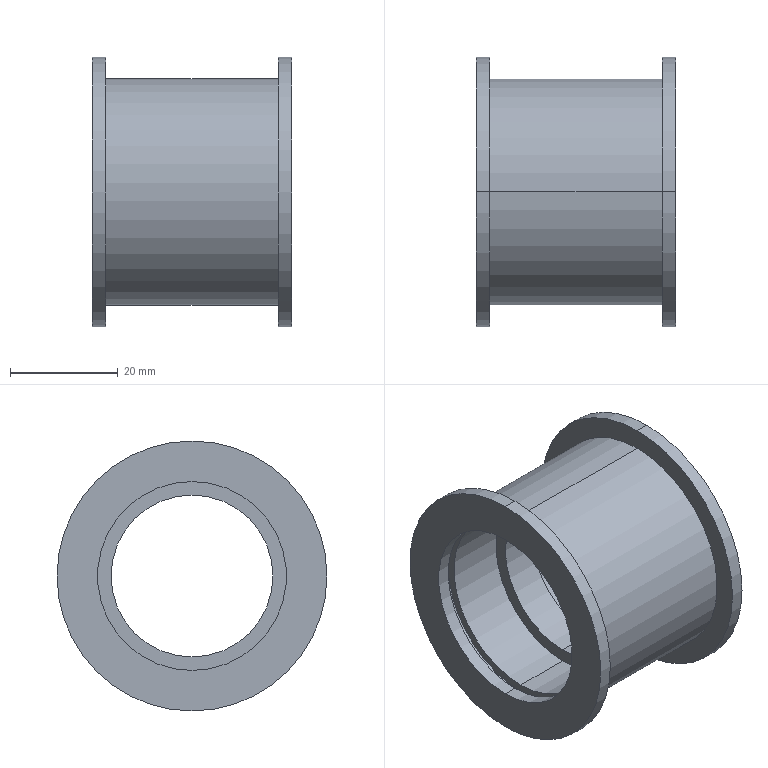Part | SolidWorks | features ICE 5, Fillet 2, MirrorPattern 2, CirPattern 1, Extrusion 1, RevCut 1 | 1 solid | 30 faces | box 37 x 50 x 50 mm | volume 19824 mm3 | cylinder 20 | plane 10 | commonest cylinder face diameters 35 x8 38 x4 50 x4 30 x2 42 x2
STEP:
#1=CARTESIAN_POINT('',(16.,0.,-19.));
#2=VERTEX_POINT('',#1);
#3=CARTESIAN_POINT('',(16.,0.,19.));
#4=VERTEX_POINT('',#3);
#5=CARTESIAN_POINT('',(16.,0.,0.));
#6=DIRECTION('',(1.,0.,0.));
#7=DIRECTION('',(0.,0.,-1.));
#8=AXIS2_PLACEMENT_3D('',#5,#6,#7);
#9=CIRCLE('',#8,19.);
#10=EDGE_CURVE('',#2,#4,#9,.T.);
#11=ORIENTED_EDGE('',*,*,#10,.T.);
#12=CARTESIAN_POINT('',(14.5,0.,19.));
#13=VERTEX_POINT('',#12);
#14=CARTESIAN_POINT('',(0.,0.,19.));
#15=DIRECTION('',(-1.,0.,0.));
#16=VECTOR('',#15,1000.);
#17=LINE('',#14,#16);
#18=EDGE_CURVE('',#4,#13,#17,.T.);
#19=ORIENTED_EDGE('',*,*,#18,.T.);
#20=CARTESIAN_POINT('',(14.5,0.,-19.));
#21=VERTEX_POINT('',#20);
#22=CARTESIAN_POINT('',(14.5,0.,0.));
#23=DIRECTION('',(1.,0.,0.));
#24=DIRECTION('',(0.,0.,-1.));
#25=AXIS2_PLACEMENT_3D('',#22,#23,#24);
#26=CIRCLE('',#25,19.);
#27=EDGE_CURVE('',#21,#13,#26,.T.);
#28=ORIENTED_EDGE('',*,*,#27,.F.);
#29=CARTESIAN_POINT('',(0.,0.,-19.));
#30=DIRECTION('',(-1.,0.,0.));
#31=VECTOR('',#30,1000.);
#32=LINE('',#29,#31);
#33=EDGE_CURVE('',#2,#21,#32,.T.);
#34=ORIENTED_EDGE('',*,*,#33,.F.);
#35=EDGE_LOOP('',(#11,#19,#28,#34));
#36=FACE_OUTER_BOUND('',#35,.T.);
#37=CARTESIAN_POINT('',(0.,0.,0.));
#38=DIRECTION('',(-1.,0.,0.));
#39=DIRECTION('',(0.,0.,-1.));
#40=AXIS2_PLACEMENT_3D('',#37,#38,#39);
#41=CYLINDRICAL_SURFACE('',#40,19.);
#42=ADVANCED_FACE('',(#36),#41,.F.);
#43=CARTESIAN_POINT('',(3.5,0.,-17.5));
#44=VERTEX_POINT('',#43);
#45=CARTESIAN_POINT('',(3.5,0.,17.5));
#46=VERTEX_POINT('',#45);
#47=CARTESIAN_POINT('',(3.5,0.,0.));
#48=DIRECTION('',(-1.,0.,0.));
#49=DIRECTION('',(0.,0.,1.));
#50=AXIS2_PLACEMENT_3D('',#47,#48,#49);
#51=CIRCLE('',#50,17.5);
#52=EDGE_CURVE('',#44,#46,#51,.T.);
#53=ORIENTED_EDGE('',*,*,#52,.T.);
#54=CARTESIAN_POINT('',(14.5,0.,17.5));
#55=VERTEX_POINT('',#54);
#56=CARTESIAN_POINT('',(3.5,0.,17.5));
#57=DIRECTION('',(1.,0.,0.));
#58=VECTOR('',#57,1000.);
#59=LINE('',#56,#58);
#60=EDGE_CURVE('',#46,#55,#59,.T.);
#61=ORIENTED_EDGE('',*,*,#60,.T.);
#62=CARTESIAN_POINT('',(14.5,0.,-17.5));
#63=VERTEX_POINT('',#62);
#64=CARTESIAN_POINT('',(14.5,0.,0.));
#65=DIRECTION('',(1.,0.,0.));
#66=DIRECTION('',(0.,0.,-1.));
#67=AXIS2_PLACEMENT_3D('',#64,#65,#66);
#68=CIRCLE('',#67,17.5);
#69=EDGE_CURVE('',#55,#63,#68,.T.);
#70=ORIENTED_EDGE('',*,*,#69,.T.);
#71=CARTESIAN_POINT('',(3.5,0.,-17.5));
#72=DIRECTION('',(1.,0.,0.));
#73=VECTOR('',#72,1000.);
#74=LINE('',#71,#73);
#75=EDGE_CURVE('',#44,#63,#74,.T.);
#76=ORIENTED_EDGE('',*,*,#75,.F.);
#77=EDGE_LOOP('',(#53,#61,#70,#76));
#78=FACE_OUTER_BOUND('',#77,.T.);
#79=CARTESIAN_POINT('',(3.5,0.,0.));
#80=DIRECTION('',(1.,0.,0.));
#81=DIRECTION('',(0.,0.,-1.));
#82=AXIS2_PLACEMENT_3D('',#79,#80,#81);
#83=CYLINDRICAL_SURFACE('',#82,17.5);
#84=ADVANCED_FACE('',(#78),#83,.F.);
#85=CARTESIAN_POINT('',(-16.,0.,19.));
#86=VERTEX_POINT('',#85);
#87=CARTESIAN_POINT('',(-16.,0.,-19.));
#88=VERTEX_POINT('',#87);
#89=CARTESIAN_POINT('',(-16.,0.,0.));
#90=DIRECTION('',(1.,0.,0.));
#91=DIRECTION('',(0.,0.,-1.));
#92=AXIS2_PLACEMENT_3D('',#89,#90,#91);
#93=CIRCLE('',#92,19.);
#94=EDGE_CURVE('',#86,#88,#93,.T.);
#95=ORIENTED_EDGE('',*,*,#94,.F.);
#96=CARTESIAN_POINT('',(-14.5,0.,19.));
#97=VERTEX_POINT('',#96);
#98=CARTESIAN_POINT('',(0.,0.,19.));
#99=DIRECTION('',(1.,0.,0.));
#100=VECTOR('',#99,1000.);
#101=LINE('',#98,#100);
#102=EDGE_CURVE('',#86,#97,#101,.T.);
#103=ORIENTED_EDGE('',*,*,#102,.T.);
#104=CARTESIAN_POINT('',(-14.5,0.,-19.));
#105=VERTEX_POINT('',#104);
#106=CARTESIAN_POINT('',(-14.5,0.,0.));
#107=DIRECTION('',(1.,0.,0.));
#108=DIRECTION('',(0.,0.,-1.));
#109=AXIS2_PLACEMENT_3D('',#106,#107,#108);
#110=CIRCLE('',#109,19.);
#111=EDGE_CURVE('',#97,#105,#110,.T.);
#112=ORIENTED_EDGE('',*,*,#111,.T.);
#113=CARTESIAN_POINT('',(0.,0.,-19.));
#114=DIRECTION('',(1.,0.,0.));
#115=VECTOR('',#114,1000.);
#116=LINE('',#113,#115);
#117=EDGE_CURVE('',#88,#105,#116,.T.);
#118=ORIENTED_EDGE('',*,*,#117,.F.);
#119=EDGE_LOOP('',(#95,#103,#112,#118));
#120=FACE_OUTER_BOUND('',#119,.T.);
#121=CARTESIAN_POINT('',(0.,0.,0.));
#122=DIRECTION('',(1.,0.,0.));
#123=DIRECTION('',(0.,0.,-1.));
#124=AXIS2_PLACEMENT_3D('',#121,#122,#123);
#125=CYLINDRICAL_SURFACE('',#124,19.);
#126=ADVANCED_FACE('',(#120),#125,.F.);
#127=CARTESIAN_POINT('',(-3.5,0.,-17.5));
#128=VERTEX_POINT('',#127);
#129=CARTESIAN_POINT('',(-3.5,0.,17.5));
#130=VERTEX_POINT('',#129);
#131=CARTESIAN_POINT('',(-3.5,0.,0.));
#132=DIRECTION('',(-1.,0.,0.));
#133=DIRECTION('',(0.,0.,1.));
#134=AXIS2_PLACEMENT_3D('',#131,#132,#133);
#135=CIRCLE('',#134,17.5);
#136=EDGE_CURVE('',#128,#130,#135,.T.);
#137=ORIENTED_EDGE('',*,*,#136,.F.);
#138=CARTESIAN_POINT('',(-14.5,0.,-17.5));
#139=VERTEX_POINT('',#138);
#140=CARTESIAN_POINT('',(-3.5,0.,-17.5));
#141=DIRECTION('',(-1.,0.,0.));
#142=VECTOR('',#141,1000.);
#143=LINE('',#140,#142);
#144=EDGE_CURVE('',#128,#139,#143,.T.);
#145=ORIENTED_EDGE('',*,*,#144,.T.);
#146=CARTESIAN_POINT('',(-14.5,0.,17.5));
#147=VERTEX_POINT('',#146);
#148=CARTESIAN_POINT('',(-14.5,0.,0.));
#149=DIRECTION('',(1.,0.,0.));
#150=DIRECTION('',(0.,0.,-1.));
#151=AXIS2_PLACEMENT_3D('',#148,#149,#150);
#152=CIRCLE('',#151,17.5);
#153=EDGE_CURVE('',#147,#139,#152,.T.);
#154=ORIENTED_EDGE('',*,*,#153,.F.);
#155=CARTESIAN_POINT('',(-3.5,0.,17.5));
#156=DIRECTION('',(-1.,0.,0.));
#157=VECTOR('',#156,1000.);
#158=LINE('',#155,#157);
#159=EDGE_CURVE('',#130,#147,#158,.T.);
#160=ORIENTED_EDGE('',*,*,#159,.F.);
#161=EDGE_LOOP('',(#137,#145,#154,#160));
#162=FACE_OUTER_BOUND('',#161,.T.);
#163=CARTESIAN_POINT('',(-3.5,0.,0.));
#164=DIRECTION('',(-1.,0.,0.));
#165=DIRECTION('',(0.,0.,1.));
#166=AXIS2_PLACEMENT_3D('',#163,#164,#165);
#167=CYLINDRICAL_SURFACE('',#166,17.5);
#168=ADVANCED_FACE('',(#162),#167,.F.);
#169=CARTESIAN_POINT('',(-18.5,0.,-25.));
#170=VERTEX_POINT('',#169);
#171=CARTESIAN_POINT('',(-18.5,0.,25.));
#172=VERTEX_POINT('',#171);
#173=CARTESIAN_POINT('',(-18.5,0.,0.));
#174=DIRECTION('',(1.,0.,0.));
#175=DIRECTION('',(0.,0.,-1.));
#176=AXIS2_PLACEMENT_3D('',#173,#174,#175);
#177=CIRCLE('',#176,25.);
#178=EDGE_CURVE('',#170,#172,#177,.T.);
#179=ORIENTED_EDGE('',*,*,#178,.T.);
#180=CARTESIAN_POINT('',(-16.,0.,25.));
#181=VERTEX_POINT('',#180);
#182=CARTESIAN_POINT('',(-17.5,0.,25.));
#183=DIRECTION('',(1.,0.,0.));
#184=VECTOR('',#183,1000.);
#185=LINE('',#182,#184);
#186=EDGE_CURVE('',#172,#181,#185,.T.);
#187=ORIENTED_EDGE('',*,*,#186,.T.);
#188=CARTESIAN_POINT('',(-16.,0.,-25.));
#189=VERTEX_POINT('',#188);
#190=CARTESIAN_POINT('',(-16.,0.,0.));
#191=DIRECTION('',(1.,0.,0.));
#192=DIRECTION('',(0.,0.,-1.));
#193=AXIS2_PLACEMENT_3D('',#190,#191,#192);
#194=CIRCLE('',#193,25.);
#195=EDGE_CURVE('',#189,#181,#194,.T.);
#196=ORIENTED_EDGE('',*,*,#195,.F.);
#197=CARTESIAN_POINT('',(-17.5,0.,-25.));
#198=DIRECTION('',(1.,0.,0.));
#199=VECTOR('',#198,1000.);
#200=LINE('',#197,#199);
#201=EDGE_CURVE('',#170,#189,#200,.T.);
#202=ORIENTED_EDGE('',*,*,#201,.F.);
#203=EDGE_LOOP('',(#179,#187,#196,#202));
#204=FACE_OUTER_BOUND('',#203,.T.);
#205=CARTESIAN_POINT('',(-17.5,0.,0.));
#206=DIRECTION('',(1.,0.,0.));
#207=DIRECTION('',(0.,0.,-1.));
#208=AXIS2_PLACEMENT_3D('',#205,#206,#207);
#209=CYLINDRICAL_SURFACE('',#208,25.);
#210=ADVANCED_FACE('',(#204),#209,.T.);
#211=CARTESIAN_POINT('',(18.5,0.,-25.));
#212=VERTEX_POINT('',#211);
#213=CARTESIAN_POINT('',(18.5,0.,25.));
#214=VERTEX_POINT('',#213);
#215=CARTESIAN_POINT('',(18.5,0.,0.));
#216=DIRECTION('',(1.,0.,0.));
#217=DIRECTION('',(0.,0.,-1.));
#218=AXIS2_PLACEMENT_3D('',#215,#216,#217);
#219=CIRCLE('',#218,25.);
#220=EDGE_CURVE('',#212,#214,#219,.T.);
#221=ORIENTED_EDGE('',*,*,#220,.F.);
#222=CARTESIAN_POINT('',(16.,0.,-25.));
#223=VERTEX_POINT('',#222);
#224=CARTESIAN_POINT('',(17.5,0.,-25.));
#225=DIRECTION('',(-1.,0.,0.));
#226=VECTOR('',#225,1000.);
#227=LINE('',#224,#226);
#228=EDGE_CURVE('',#212,#223,#227,.T.);
#229=ORIENTED_EDGE('',*,*,#228,.T.);
#230=CARTESIAN_POINT('',(16.,0.,25.));
#231=VERTEX_POINT('',#230);
#232=CARTESIAN_POINT('',(16.,0.,0.));
#233=DIRECTION('',(1.,0.,0.));
#234=DIRECTION('',(0.,0.,-1.));
#235=AXIS2_PLACEMENT_3D('',#232,#233,#234);
#236=CIRCLE('',#235,25.);
#237=EDGE_CURVE('',#223,#231,#236,.T.);
#238=ORIENTED_EDGE('',*,*,#237,.T.);
#239=CARTESIAN_POINT('',(17.5,0.,25.));
#240=DIRECTION('',(-1.,0.,0.));
#241=VECTOR('',#240,1000.);
#242=LINE('',#239,#241);
#243=EDGE_CURVE('',#214,#231,#242,.T.);
#244=ORIENTED_EDGE('',*,*,#243,.F.);
#245=EDGE_LOOP('',(#221,#229,#238,#244));
#246=FACE_OUTER_BOUND('',#245,.T.);
#247=CARTESIAN_POINT('',(17.5,0.,0.));
#248=DIRECTION('',(-1.,0.,0.));
#249=DIRECTION('',(0.,0.,1.));
#250=AXIS2_PLACEMENT_3D('',#247,#248,#249);
#251=CYLINDRICAL_SURFACE('',#250,25.);
#252=ADVANCED_FACE('',(#246),#251,.T.);
#253=CARTESIAN_POINT('',(16.,0.,-21.));
#254=VERTEX_POINT('',#253);
#255=CARTESIAN_POINT('',(16.,0.,21.));
#256=VERTEX_POINT('',#255);
#257=CARTESIAN_POINT('',(16.,0.,0.));
#258=DIRECTION('',(1.,0.,0.));
#259=DIRECTION('',(0.,0.,-1.));
#260=AXIS2_PLACEMENT_3D('',#257,#258,#259);
#261=CIRCLE('',#260,21.);
#262=EDGE_CURVE('',#254,#256,#261,.T.);
#263=ORIENTED_EDGE('',*,*,#262,.F.);
#264=CARTESIAN_POINT('',(-16.,0.,-21.));
#265=VERTEX_POINT('',#264);
#266=CARTESIAN_POINT('',(16.,0.,-21.));
#267=DIRECTION('',(-1.,0.,0.));
#268=VECTOR('',#267,1000.);
#269=LINE('',#266,#268);
#270=EDGE_CURVE('',#254,#265,#269,.T.);
#271=ORIENTED_EDGE('',*,*,#270,.T.);
#272=CARTESIAN_POINT('',(-16.,0.,21.));
#273=VERTEX_POINT('',#272);
#274=CARTESIAN_POINT('',(-16.,0.,0.));
#275=DIRECTION('',(-1.,0.,0.));
#276=DIRECTION('',(0.,0.,1.));
#277=AXIS2_PLACEMENT_3D('',#274,#275,#276);
#278=CIRCLE('',#277,21.);
#279=EDGE_CURVE('',#273,#265,#278,.T.);
#280=ORIENTED_EDGE('',*,*,#279,.F.);
#281=CARTESIAN_POINT('',(16.,0.,21.));
#282=DIRECTION('',(-1.,0.,0.));
#283=VECTOR('',#282,1000.);
#284=LINE('',#281,#283);
#285=EDGE_CURVE('',#256,#273,#284,.T.);
#286=ORIENTED_EDGE('',*,*,#285,.F.);
#287=EDGE_LOOP('',(#263,#271,#280,#286));
#288=FACE_OUTER_BOUND('',#287,.T.);
#289=CARTESIAN_POINT('',(16.,0.,0.));
#290=DIRECTION('',(-1.,0.,0.));
#291=DIRECTION('',(0.,0.,1.));
#292=AXIS2_PLACEMENT_3D('',#289,#290,#291);
#293=CYLINDRICAL_SURFACE('',#292,21.);
#294=ADVANCED_FACE('',(#288),#293,.T.);
#295=CARTESIAN_POINT('',(-16.,0.,17.5));
#296=VERTEX_POINT('',#295);
#297=CARTESIAN_POINT('',(-16.,0.,-17.5));
#298=VERTEX_POINT('',#297);
#299=CARTESIAN_POINT('',(-16.,0.,0.));
#300=DIRECTION('',(1.,0.,0.));
#301=DIRECTION('',(0.,0.,-1.));
#302=AXIS2_PLACEMENT_3D('',#299,#300,#301);
#303=CIRCLE('',#302,17.5);
#304=EDGE_CURVE('',#296,#298,#303,.T.);
#305=ORIENTED_EDGE('',*,*,#304,.T.);
#306=CARTESIAN_POINT('',(-18.5,0.,-17.5));
#307=VERTEX_POINT('',#306);
#308=CARTESIAN_POINT('',(-3.5,0.,-17.5));
#309=DIRECTION('',(-1.,0.,0.));
#310=VECTOR('',#309,1000.);
#311=LINE('',#308,#310);
#312=EDGE_CURVE('',#298,#307,#311,.T.);
#313=ORIENTED_EDGE('',*,*,#312,.T.);
#314=CARTESIAN_POINT('',(-18.5,0.,17.5));
#315=VERTEX_POINT('',#314);
#316=CARTESIAN_POINT('',(-18.5,0.,0.));
#317=DIRECTION('',(-1.,0.,0.));
#318=DIRECTION('',(0.,0.,1.));
#319=AXIS2_PLACEMENT_3D('',#316,#317,#318);
#320=CIRCLE('',#319,17.5);
#321=EDGE_CURVE('',#307,#315,#320,.T.);
#322=ORIENTED_EDGE('',*,*,#321,.T.);
#323=CARTESIAN_POINT('',(-3.5,0.,17.5));
#324=DIRECTION('',(-1.,0.,0.));
#325=VECTOR('',#324,1000.);
#326=LINE('',#323,#325);
#327=EDGE_CURVE('',#296,#315,#326,.T.);
#328=ORIENTED_EDGE('',*,*,#327,.F.);
#329=EDGE_LOOP('',(#305,#313,#322,#328));
#330=FACE_OUTER_BOUND('',#329,.T.);
#331=CARTESIAN_POINT('',(-3.5,0.,0.));
#332=DIRECTION('',(-1.,0.,0.));
#333=DIRECTION('',(0.,0.,1.));
#334=AXIS2_PLACEMENT_3D('',#331,#332,#333);
#335=CYLINDRICAL_SURFACE('',#334,17.5);
#336=ADVANCED_FACE('',(#330),#335,.F.);
#337=CARTESIAN_POINT('',(3.5,0.,-15.));
#338=VERTEX_POINT('',#337);
#339=CARTESIAN_POINT('',(3.5,0.,15.));
#340=VERTEX_POINT('',#339);
#341=CARTESIAN_POINT('',(3.5,0.,0.));
#342=DIRECTION('',(-1.,0.,0.));
#343=DIRECTION('',(0.,0.,-1.));
#344=AXIS2_PLACEMENT_3D('',#341,#342,#343);
#345=CIRCLE('',#344,15.);
#346=EDGE_CURVE('',#338,#340,#345,.T.);
#347=ORIENTED_EDGE('',*,*,#346,.F.);
#348=CARTESIAN_POINT('',(-3.5,0.,-15.));
#349=VERTEX_POINT('',#348);
#350=CARTESIAN_POINT('',(18.5,0.,-15.));
#351=DIRECTION('',(-1.,0.,0.));
#352=VECTOR('',#351,1000.);
#353=LINE('',#350,#352);
#354=EDGE_CURVE('',#338,#349,#353,.T.);
#355=ORIENTED_EDGE('',*,*,#354,.T.);
#356=CARTESIAN_POINT('',(-3.5,0.,15.));
#357=VERTEX_POINT('',#356);
#358=CARTESIAN_POINT('',(-3.5,0.,0.));
#359=DIRECTION('',(1.,0.,0.));
#360=DIRECTION('',(0.,0.,1.));
#361=AXIS2_PLACEMENT_3D('',#358,#359,#360);
#362=CIRCLE('',#361,15.);
#363=EDGE_CURVE('',#357,#349,#362,.T.);
#364=ORIENTED_EDGE('',*,*,#363,.F.);
#365=CARTESIAN_POINT('',(18.5,0.,15.));
#366=DIRECTION('',(-1.,0.,0.));
#367=VECTOR('',#366,1000.);
#368=LINE('',#365,#367);
#369=EDGE_CURVE('',#340,#357,#368,.T.);
#370=ORIENTED_EDGE('',*,*,#369,.F.);
#371=EDGE_LOOP('',(#347,#355,#364,#370));
#372=FACE_OUTER_BOUND('',#371,.T.);
#373=CARTESIAN_POINT('',(18.5,0.,0.));
#374=DIRECTION('',(-1.,0.,0.));
#375=DIRECTION('',(0.,0.,1.));
#376=AXIS2_PLACEMENT_3D('',#373,#374,#375);
#377=CYLINDRICAL_SURFACE('',#376,15.);
#378=ADVANCED_FACE('',(#372),#377,.F.);
#379=CARTESIAN_POINT('',(16.,0.,17.5));
#380=VERTEX_POINT('',#379);
#381=CARTESIAN_POINT('',(16.,0.,-17.5));
#382=VERTEX_POINT('',#381);
#383=CARTESIAN_POINT('',(16.,0.,0.));
#384=DIRECTION('',(1.,0.,0.));
#385=DIRECTION('',(0.,0.,-1.));
#386=AXIS2_PLACEMENT_3D('',#383,#384,#385);
#387=CIRCLE('',#386,17.5);
#388=EDGE_CURVE('',#380,#382,#387,.T.);
#389=ORIENTED_EDGE('',*,*,#388,.F.);
#390=CARTESIAN_POINT('',(18.5,0.,17.5));
#391=VERTEX_POINT('',#390);
#392=CARTESIAN_POINT('',(3.5,0.,17.5));
#393=DIRECTION('',(1.,0.,0.));
#394=VECTOR('',#393,1000.);
#395=LINE('',#392,#394);
#396=EDGE_CURVE('',#380,#391,#395,.T.);
#397=ORIENTED_EDGE('',*,*,#396,.T.);
#398=CARTESIAN_POINT('',(18.5,0.,-17.5));
#399=VERTEX_POINT('',#398);
#400=CARTESIAN_POINT('',(18.5,0.,0.));
#401=DIRECTION('',(-1.,0.,0.));
#402=DIRECTION('',(0.,0.,1.));
#403=AXIS2_PLACEMENT_3D('',#400,#401,#402);
#404=CIRCLE('',#403,17.5);
#405=EDGE_CURVE('',#399,#391,#404,.T.);
#406=ORIENTED_EDGE('',*,*,#405,.F.);
#407=CARTESIAN_POINT('',(3.5,0.,-17.5));
#408=DIRECTION('',(1.,0.,0.));
#409=VECTOR('',#408,1000.);
#410=LINE('',#407,#409);
#411=EDGE_CURVE('',#382,#399,#410,.T.);
#412=ORIENTED_EDGE('',*,*,#411,.F.);
#413=EDGE_LOOP('',(#389,#397,#406,#412));
#414=FACE_OUTER_BOUND('',#413,.T.);
#415=CARTESIAN_POINT('',(3.5,0.,0.));
#416=DIRECTION('',(1.,0.,0.));
#417=DIRECTION('',(0.,0.,-1.));
#418=AXIS2_PLACEMENT_3D('',#415,#416,#417);
#419=CYLINDRICAL_SURFACE('',#418,17.5);
#420=ADVANCED_FACE('',(#414),#419,.F.);
#421=ORIENTED_EDGE('',*,*,#396,.F.);
#422=CARTESIAN_POINT('',(16.,0.,0.));
#423=DIRECTION('',(1.,0.,0.));
#424=DIRECTION('',(0.,0.,-1.));
#425=AXIS2_PLACEMENT_3D('',#422,#423,#424);
#426=CIRCLE('',#425,17.5);
#427=EDGE_CURVE('',#382,#380,#426,.T.);
#428=ORIENTED_EDGE('',*,*,#427,.F.);
#429=ORIENTED_EDGE('',*,*,#411,.T.);
#430=CARTESIAN_POINT('',(18.5,0.,0.));
#431=DIRECTION('',(-1.,0.,0.));
#432=DIRECTION('',(0.,0.,1.));
#433=AXIS2_PLACEMENT_3D('',#430,#431,#432);
#434=CIRCLE('',#433,17.5);
#435=EDGE_CURVE('',#391,#399,#434,.T.);
#436=ORIENTED_EDGE('',*,*,#435,.F.);
#437=EDGE_LOOP('',(#421,#428,#429,#436));
#438=FACE_OUTER_BOUND('',#437,.T.);
#439=CARTESIAN_POINT('',(3.5,0.,0.));
#440=DIRECTION('',(1.,0.,0.));
#441=DIRECTION('',(0.,0.,-1.));
#442=AXIS2_PLACEMENT_3D('',#439,#440,#441);
#443=CYLINDRICAL_SURFACE('',#442,17.5);
#444=ADVANCED_FACE('',(#438),#443,.F.);
#445=ORIENTED_EDGE('',*,*,#354,.F.);
#446=CARTESIAN_POINT('',(3.5,0.,0.));
#447=DIRECTION('',(-1.,0.,0.));
#448=DIRECTION('',(0.,0.,-1.));
#449=AXIS2_PLACEMENT_3D('',#446,#447,#448);
#450=CIRCLE('',#449,15.);
#451=EDGE_CURVE('',#340,#338,#450,.T.);
#452=ORIENTED_EDGE('',*,*,#451,.F.);
#453=ORIENTED_EDGE('',*,*,#369,.T.);
#454=CARTESIAN_POINT('',(-3.5,0.,0.));
#455=DIRECTION('',(1.,0.,0.));
#456=DIRECTION('',(0.,0.,1.));
#457=AXIS2_PLACEMENT_3D('',#454,#455,#456);
#458=CIRCLE('',#457,15.);
#459=EDGE_CURVE('',#349,#357,#458,.T.);
#460=ORIENTED_EDGE('',*,*,#459,.F.);
#461=EDGE_LOOP('',(#445,#452,#453,#460));
#462=FACE_OUTER_BOUND('',#461,.T.);
#463=CARTESIAN_POINT('',(18.5,0.,0.));
#464=DIRECTION('',(-1.,0.,0.));
#465=DIRECTION('',(0.,0.,1.));
#466=AXIS2_PLACEMENT_3D('',#463,#464,#465);
#467=CYLINDRICAL_SURFACE('',#466,15.);
#468=ADVANCED_FACE('',(#462),#467,.F.);
#469=CARTESIAN_POINT('',(18.5,0.,0.));
#470=DIRECTION('',(1.,0.,0.));
#471=DIRECTION('',(0.,0.,-1.));
#472=AXIS2_PLACEMENT_3D('',#469,#470,#471);
#473=CIRCLE('',#472,25.);
#474=EDGE_CURVE('',#214,#212,#473,.T.);
#475=ORIENTED_EDGE('',*,*,#474,.T.);
#476=ORIENTED_EDGE('',*,*,#220,.T.);
#477=EDGE_LOOP('',(#475,#476));
#478=FACE_OUTER_BOUND('',#477,.T.);
#479=ORIENTED_EDGE('',*,*,#405,.T.);
#480=ORIENTED_EDGE('',*,*,#435,.T.);
#481=EDGE_LOOP('',(#479,#480));
#482=FACE_BOUND('',#481,.T.);
#483=CARTESIAN_POINT('',(18.5,0.,0.));
#484=DIRECTION('',(1.,0.,0.));
#485=DIRECTION('',(0.,0.,-1.));
#486=AXIS2_PLACEMENT_3D('',#483,#484,#485);
#487=PLANE('',#486);
#488=ADVANCED_FACE('',(#478,#482),#487,.T.);
#489=ORIENTED_EDGE('',*,*,#312,.F.);
#490=CARTESIAN_POINT('',(-16.,0.,0.));
#491=DIRECTION('',(1.,0.,0.));
#492=DIRECTION('',(0.,0.,-1.));
#493=AXIS2_PLACEMENT_3D('',#490,#491,#492);
#494=CIRCLE('',#493,17.5);
#495=EDGE_CURVE('',#298,#296,#494,.T.);
#496=ORIENTED_EDGE('',*,*,#495,.T.);
#497=ORIENTED_EDGE('',*,*,#327,.T.);
#498=CARTESIAN_POINT('',(-18.5,0.,0.));
#499=DIRECTION('',(-1.,0.,0.));
#500=DIRECTION('',(0.,0.,1.));
#501=AXIS2_PLACEMENT_3D('',#498,#499,#500);
#502=CIRCLE('',#501,17.5);
#503=EDGE_CURVE('',#315,#307,#502,.T.);
#504=ORIENTED_EDGE('',*,*,#503,.T.);
#505=EDGE_LOOP('',(#489,#496,#497,#504));
#506=FACE_OUTER_BOUND('',#505,.T.);
#507=CARTESIAN_POINT('',(-3.5,0.,0.));
#508=DIRECTION('',(-1.,0.,0.));
#509=DIRECTION('',(0.,0.,1.));
#510=AXIS2_PLACEMENT_3D('',#507,#508,#509);
#511=CYLINDRICAL_SURFACE('',#510,17.5);
#512=ADVANCED_FACE('',(#506),#511,.F.);
#513=ORIENTED_EDGE('',*,*,#270,.F.);
#514=CARTESIAN_POINT('',(16.,0.,0.));
#515=DIRECTION('',(1.,0.,0.));
#516=DIRECTION('',(0.,0.,-1.));
#517=AXIS2_PLACEMENT_3D('',#514,#515,#516);
#518=CIRCLE('',#517,21.);
#519=EDGE_CURVE('',#256,#254,#518,.T.);
#520=ORIENTED_EDGE('',*,*,#519,.F.);
#521=ORIENTED_EDGE('',*,*,#285,.T.);
#522=CARTESIAN_POINT('',(-16.,0.,0.));
#523=DIRECTION('',(-1.,0.,0.));
#524=DIRECTION('',(0.,0.,1.));
#525=AXIS2_PLACEMENT_3D('',#522,#523,#524);
#526=CIRCLE('',#525,21.);
#527=EDGE_CURVE('',#265,#273,#526,.T.);
#528=ORIENTED_EDGE('',*,*,#527,.F.);
#529=EDGE_LOOP('',(#513,#520,#521,#528));
#530=FACE_OUTER_BOUND('',#529,.T.);
#531=CARTESIAN_POINT('',(16.,0.,0.));
#532=DIRECTION('',(-1.,0.,0.));
#533=DIRECTION('',(0.,0.,1.));
#534=AXIS2_PLACEMENT_3D('',#531,#532,#533);
#535=CYLINDRICAL_SURFACE('',#534,21.);
#536=ADVANCED_FACE('',(#530),#535,.T.);
#537=CARTESIAN_POINT('',(16.,0.,0.));
#538=DIRECTION('',(1.,0.,0.));
#539=DIRECTION('',(0.,0.,-1.));
#540=AXIS2_PLACEMENT_3D('',#537,#538,#539);
#541=CIRCLE('',#540,25.);
#542=EDGE_CURVE('',#231,#223,#541,.T.);
#543=ORIENTED_EDGE('',*,*,#542,.F.);
#544=ORIENTED_EDGE('',*,*,#237,.F.);
#545=EDGE_LOOP('',(#543,#544));
#546=FACE_OUTER_BOUND('',#545,.T.);
#547=ORIENTED_EDGE('',*,*,#519,.T.);
#548=ORIENTED_EDGE('',*,*,#262,.T.);
#549=EDGE_LOOP('',(#547,#548));
#550=FACE_BOUND('',#549,.T.);
#551=CARTESIAN_POINT('',(16.,0.,0.));
#552=DIRECTION('',(1.,0.,0.));
#553=DIRECTION('',(0.,0.,-1.));
#554=AXIS2_PLACEMENT_3D('',#551,#552,#553);
#555=PLANE('',#554);
#556=ADVANCED_FACE('',(#546,#550),#555,.F.);
#557=ORIENTED_EDGE('',*,*,#228,.F.);
#558=ORIENTED_EDGE('',*,*,#474,.F.);
#559=ORIENTED_EDGE('',*,*,#243,.T.);
#560=ORIENTED_EDGE('',*,*,#542,.T.);
#561=EDGE_LOOP('',(#557,#558,#559,#560));
#562=FACE_OUTER_BOUND('',#561,.T.);
#563=CARTESIAN_POINT('',(17.5,0.,0.));
#564=DIRECTION('',(-1.,0.,0.));
#565=DIRECTION('',(0.,0.,1.));
#566=AXIS2_PLACEMENT_3D('',#563,#564,#565);
#567=CYLINDRICAL_SURFACE('',#566,25.);
#568=ADVANCED_FACE('',(#562),#567,.T.);
#569=ORIENTED_EDGE('',*,*,#195,.T.);
#570=CARTESIAN_POINT('',(-16.,0.,0.));
#571=DIRECTION('',(1.,0.,0.));
#572=DIRECTION('',(0.,0.,-1.));
#573=AXIS2_PLACEMENT_3D('',#570,#571,#572);
#574=CIRCLE('',#573,25.);
#575=EDGE_CURVE('',#181,#189,#574,.T.);
#576=ORIENTED_EDGE('',*,*,#575,.T.);
#577=EDGE_LOOP('',(#569,#576));
#578=FACE_OUTER_BOUND('',#577,.T.);
#579=ORIENTED_EDGE('',*,*,#279,.T.);
#580=ORIENTED_EDGE('',*,*,#527,.T.);
#581=EDGE_LOOP('',(#579,#580));
#582=FACE_BOUND('',#581,.T.);
#583=CARTESIAN_POINT('',(-16.,0.,0.));
#584=DIRECTION('',(-1.,0.,0.));
#585=DIRECTION('',(0.,0.,-1.));
#586=AXIS2_PLACEMENT_3D('',#583,#584,#585);
#587=PLANE('',#586);
#588=ADVANCED_FACE('',(#578,#582),#587,.F.);
#589=ORIENTED_EDGE('',*,*,#186,.F.);
#590=CARTESIAN_POINT('',(-18.5,0.,0.));
#591=DIRECTION('',(1.,0.,0.));
#592=DIRECTION('',(0.,0.,-1.));
#593=AXIS2_PLACEMENT_3D('',#590,#591,#592);
#594=CIRCLE('',#593,25.);
#595=EDGE_CURVE('',#172,#170,#594,.T.);
#596=ORIENTED_EDGE('',*,*,#595,.T.);
#597=ORIENTED_EDGE('',*,*,#201,.T.);
#598=ORIENTED_EDGE('',*,*,#575,.F.);
#599=EDGE_LOOP('',(#589,#596,#597,#598));
#600=FACE_OUTER_BOUND('',#599,.T.);
#601=CARTESIAN_POINT('',(-17.5,0.,0.));
#602=DIRECTION('',(1.,0.,0.));
#603=DIRECTION('',(0.,0.,-1.));
#604=AXIS2_PLACEMENT_3D('',#601,#602,#603);
#605=CYLINDRICAL_SURFACE('',#604,25.);
#606=ADVANCED_FACE('',(#600),#605,.T.);
#607=ORIENTED_EDGE('',*,*,#503,.F.);
#608=ORIENTED_EDGE('',*,*,#321,.F.);
#609=EDGE_LOOP('',(#607,#608));
#610=FACE_BOUND('',#609,.T.);
#611=ORIENTED_EDGE('',*,*,#178,.F.);
#612=ORIENTED_EDGE('',*,*,#595,.F.);
#613=EDGE_LOOP('',(#611,#612));
#614=FACE_OUTER_BOUND('',#613,.T.);
#615=CARTESIAN_POINT('',(-18.5,0.,0.));
#616=DIRECTION('',(-1.,0.,0.));
#617=DIRECTION('',(0.,0.,-1.));
#618=AXIS2_PLACEMENT_3D('',#615,#616,#617);
#619=PLANE('',#618);
#620=ADVANCED_FACE('',(#610,#614),#619,.T.);
#621=CARTESIAN_POINT('',(-3.5,0.,0.));
#622=DIRECTION('',(-1.,0.,0.));
#623=DIRECTION('',(0.,0.,1.));
#624=AXIS2_PLACEMENT_3D('',#621,#622,#623);
#625=CIRCLE('',#624,17.5);
#626=EDGE_CURVE('',#130,#128,#625,.T.);
#627=ORIENTED_EDGE('',*,*,#626,.T.);
#628=ORIENTED_EDGE('',*,*,#136,.T.);
#629=EDGE_LOOP('',(#627,#628));
#630=FACE_OUTER_BOUND('',#629,.T.);
#631=ORIENTED_EDGE('',*,*,#363,.T.);
#632=ORIENTED_EDGE('',*,*,#459,.T.);
#633=EDGE_LOOP('',(#631,#632));
#634=FACE_BOUND('',#633,.T.);
#635=CARTESIAN_POINT('',(-3.5,0.,0.));
#636=DIRECTION('',(-1.,0.,0.));
#637=DIRECTION('',(0.,0.,1.));
#638=AXIS2_PLACEMENT_3D('',#635,#636,#637);
#639=PLANE('',#638);
#640=ADVANCED_FACE('',(#630,#634),#639,.T.);
#641=ORIENTED_EDGE('',*,*,#144,.F.);
#642=ORIENTED_EDGE('',*,*,#626,.F.);
#643=ORIENTED_EDGE('',*,*,#159,.T.);
#644=CARTESIAN_POINT('',(-14.5,0.,0.));
#645=DIRECTION('',(1.,0.,0.));
#646=DIRECTION('',(0.,0.,-1.));
#647=AXIS2_PLACEMENT_3D('',#644,#645,#646);
#648=CIRCLE('',#647,17.5);
#649=EDGE_CURVE('',#139,#147,#648,.T.);
#650=ORIENTED_EDGE('',*,*,#649,.F.);
#651=EDGE_LOOP('',(#641,#642,#643,#650));
#652=FACE_OUTER_BOUND('',#651,.T.);
#653=CARTESIAN_POINT('',(-3.5,0.,0.));
#654=DIRECTION('',(-1.,0.,0.));
#655=DIRECTION('',(0.,0.,1.));
#656=AXIS2_PLACEMENT_3D('',#653,#654,#655);
#657=CYLINDRICAL_SURFACE('',#656,17.5);
#658=ADVANCED_FACE('',(#652),#657,.F.);
#659=ORIENTED_EDGE('',*,*,#304,.F.);
#660=ORIENTED_EDGE('',*,*,#495,.F.);
#661=EDGE_LOOP('',(#659,#660));
#662=FACE_BOUND('',#661,.T.);
#663=CARTESIAN_POINT('',(-16.,0.,0.));
#664=DIRECTION('',(1.,0.,0.));
#665=DIRECTION('',(0.,0.,-1.));
#666=AXIS2_PLACEMENT_3D('',#663,#664,#665);
#667=CIRCLE('',#666,19.);
#668=EDGE_CURVE('',#88,#86,#667,.T.);
#669=ORIENTED_EDGE('',*,*,#668,.T.);
#670=ORIENTED_EDGE('',*,*,#94,.T.);
#671=EDGE_LOOP('',(#669,#670));
#672=FACE_OUTER_BOUND('',#671,.T.);
#673=CARTESIAN_POINT('',(-16.,0.,-17.5));
#674=DIRECTION('',(-1.,0.,0.));
#675=DIRECTION('',(0.,0.,1.));
#676=AXIS2_PLACEMENT_3D('',#673,#674,#675);
#677=PLANE('',#676);
#678=ADVANCED_FACE('',(#662,#672),#677,.F.);
#679=ORIENTED_EDGE('',*,*,#102,.F.);
#680=ORIENTED_EDGE('',*,*,#668,.F.);
#681=ORIENTED_EDGE('',*,*,#117,.T.);
#682=CARTESIAN_POINT('',(-14.5,0.,0.));
#683=DIRECTION('',(1.,0.,0.));
#684=DIRECTION('',(0.,0.,-1.));
#685=AXIS2_PLACEMENT_3D('',#682,#683,#684);
#686=CIRCLE('',#685,19.);
#687=EDGE_CURVE('',#105,#97,#686,.T.);
#688=ORIENTED_EDGE('',*,*,#687,.T.);
#689=EDGE_LOOP('',(#679,#680,#681,#688));
#690=FACE_OUTER_BOUND('',#689,.T.);
#691=CARTESIAN_POINT('',(0.,0.,0.));
#692=DIRECTION('',(1.,0.,0.));
#693=DIRECTION('',(0.,0.,-1.));
#694=AXIS2_PLACEMENT_3D('',#691,#692,#693);
#695=CYLINDRICAL_SURFACE('',#694,19.);
#696=ADVANCED_FACE('',(#690),#695,.F.);
#697=ORIENTED_EDGE('',*,*,#687,.F.);
#698=ORIENTED_EDGE('',*,*,#111,.F.);
#699=EDGE_LOOP('',(#697,#698));
#700=FACE_OUTER_BOUND('',#699,.T.);
#701=ORIENTED_EDGE('',*,*,#153,.T.);
#702=ORIENTED_EDGE('',*,*,#649,.T.);
#703=EDGE_LOOP('',(#701,#702));
#704=FACE_BOUND('',#703,.T.);
#705=CARTESIAN_POINT('',(-14.5,0.,-17.5));
#706=DIRECTION('',(1.,0.,0.));
#707=DIRECTION('',(0.,0.,-1.));
#708=AXIS2_PLACEMENT_3D('',#705,#706,#707);
#709=PLANE('',#708);
#710=ADVANCED_FACE('',(#700,#704),#709,.F.);
#711=ORIENTED_EDGE('',*,*,#52,.F.);
#712=CARTESIAN_POINT('',(3.5,0.,0.));
#713=DIRECTION('',(-1.,0.,0.));
#714=DIRECTION('',(0.,0.,1.));
#715=AXIS2_PLACEMENT_3D('',#712,#713,#714);
#716=CIRCLE('',#715,17.5);
#717=EDGE_CURVE('',#46,#44,#716,.T.);
#718=ORIENTED_EDGE('',*,*,#717,.F.);
#719=EDGE_LOOP('',(#711,#718));
#720=FACE_OUTER_BOUND('',#719,.T.);
#721=ORIENTED_EDGE('',*,*,#451,.T.);
#722=ORIENTED_EDGE('',*,*,#346,.T.);
#723=EDGE_LOOP('',(#721,#722));
#724=FACE_BOUND('',#723,.T.);
#725=CARTESIAN_POINT('',(3.5,0.,0.));
#726=DIRECTION('',(1.,0.,0.));
#727=DIRECTION('',(0.,0.,1.));
#728=AXIS2_PLACEMENT_3D('',#725,#726,#727);
#729=PLANE('',#728);
#730=ADVANCED_FACE('',(#720,#724),#729,.T.);
#731=ORIENTED_EDGE('',*,*,#60,.F.);
#732=ORIENTED_EDGE('',*,*,#717,.T.);
#733=ORIENTED_EDGE('',*,*,#75,.T.);
#734=CARTESIAN_POINT('',(14.5,0.,0.));
#735=DIRECTION('',(1.,0.,0.));
#736=DIRECTION('',(0.,0.,-1.));
#737=AXIS2_PLACEMENT_3D('',#734,#735,#736);
#738=CIRCLE('',#737,17.5);
#739=EDGE_CURVE('',#63,#55,#738,.T.);
#740=ORIENTED_EDGE('',*,*,#739,.T.);
#741=EDGE_LOOP('',(#731,#732,#733,#740));
#742=FACE_OUTER_BOUND('',#741,.T.);
#743=CARTESIAN_POINT('',(3.5,0.,0.));
#744=DIRECTION('',(1.,0.,0.));
#745=DIRECTION('',(0.,0.,-1.));
#746=AXIS2_PLACEMENT_3D('',#743,#744,#745);
#747=CYLINDRICAL_SURFACE('',#746,17.5);
#748=ADVANCED_FACE('',(#742),#747,.F.);
#749=ORIENTED_EDGE('',*,*,#427,.T.);
#750=ORIENTED_EDGE('',*,*,#388,.T.);
#751=EDGE_LOOP('',(#749,#750));
#752=FACE_BOUND('',#751,.T.);
#753=ORIENTED_EDGE('',*,*,#10,.F.);
#754=CARTESIAN_POINT('',(16.,0.,0.));
#755=DIRECTION('',(1.,0.,0.));
#756=DIRECTION('',(0.,0.,-1.));
#757=AXIS2_PLACEMENT_3D('',#754,#755,#756);
#758=CIRCLE('',#757,19.);
#759=EDGE_CURVE('',#4,#2,#758,.T.);
#760=ORIENTED_EDGE('',*,*,#759,.F.);
#761=EDGE_LOOP('',(#753,#760));
#762=FACE_OUTER_BOUND('',#761,.T.);
#763=CARTESIAN_POINT('',(16.,0.,-17.5));
#764=DIRECTION('',(1.,0.,0.));
#765=DIRECTION('',(0.,0.,1.));
#766=AXIS2_PLACEMENT_3D('',#763,#764,#765);
#767=PLANE('',#766);
#768=ADVANCED_FACE('',(#752,#762),#767,.F.);
#769=ORIENTED_EDGE('',*,*,#18,.F.);
#770=ORIENTED_EDGE('',*,*,#759,.T.);
#771=ORIENTED_EDGE('',*,*,#33,.T.);
#772=CARTESIAN_POINT('',(14.5,0.,0.));
#773=DIRECTION('',(1.,0.,0.));
#774=DIRECTION('',(0.,0.,-1.));
#775=AXIS2_PLACEMENT_3D('',#772,#773,#774);
#776=CIRCLE('',#775,19.);
#777=EDGE_CURVE('',#13,#21,#776,.T.);
#778=ORIENTED_EDGE('',*,*,#777,.F.);
#779=EDGE_LOOP('',(#769,#770,#771,#778));
#780=FACE_OUTER_BOUND('',#779,.T.);
#781=CARTESIAN_POINT('',(0.,0.,0.));
#782=DIRECTION('',(-1.,0.,0.));
#783=DIRECTION('',(0.,0.,-1.));
#784=AXIS2_PLACEMENT_3D('',#781,#782,#783);
#785=CYLINDRICAL_SURFACE('',#784,19.);
#786=ADVANCED_FACE('',(#780),#785,.F.);
#787=ORIENTED_EDGE('',*,*,#27,.T.);
#788=ORIENTED_EDGE('',*,*,#777,.T.);
#789=EDGE_LOOP('',(#787,#788));
#790=FACE_OUTER_BOUND('',#789,.T.);
#791=ORIENTED_EDGE('',*,*,#739,.F.);
#792=ORIENTED_EDGE('',*,*,#69,.F.);
#793=EDGE_LOOP('',(#791,#792));
#794=FACE_BOUND('',#793,.T.);
#795=CARTESIAN_POINT('',(14.5,0.,-17.5));
#796=DIRECTION('',(-1.,0.,0.));
#797=DIRECTION('',(0.,0.,-1.));
#798=AXIS2_PLACEMENT_3D('',#795,#796,#797);
#799=PLANE('',#798);
#800=ADVANCED_FACE('',(#790,#794),#799,.F.);
#801=CLOSED_SHELL('',(#42,#84,#126,#168,#210,#252,#294,#336,#378,#420,#444,#468,#488,#512,#536,#556,#568,#588,#606,#620,#640,#658,#678,#696,#710,#730,#748,#768,#786,#800));
#802=MANIFOLD_SOLID_BREP('',#801);
#803=CARTESIAN_POINT('',(0.,0.,0.));
#804=DIRECTION('',(0.,0.,1.));
#805=DIRECTION('',(1.,0.,0.));
#806=AXIS2_PLACEMENT_3D('',#803,#804,#805);
#807=(LENGTH_UNIT()NAMED_UNIT(*)SI_UNIT(.MILLI.,.METRE.));
#808=UNCERTAINTY_MEASURE_WITH_UNIT(LENGTH_MEASURE(0.00001),#807,'','');
#809=(NAMED_UNIT(*)PLANE_ANGLE_UNIT()SI_UNIT($,.RADIAN.));
#810=(NAMED_UNIT(*)SI_UNIT($,.STERADIAN.)SOLID_ANGLE_UNIT());
#811=(GEOMETRIC_REPRESENTATION_CONTEXT(3)GLOBAL_UNCERTAINTY_ASSIGNED_CONTEXT((#808))GLOBAL_UNIT_ASSIGNED_CONTEXT((#807,#809,#810))REPRESENTATION_CONTEXT('',''));
#812=ADVANCED_BREP_SHAPE_REPRESENTATION('',(#802,#806),#811);